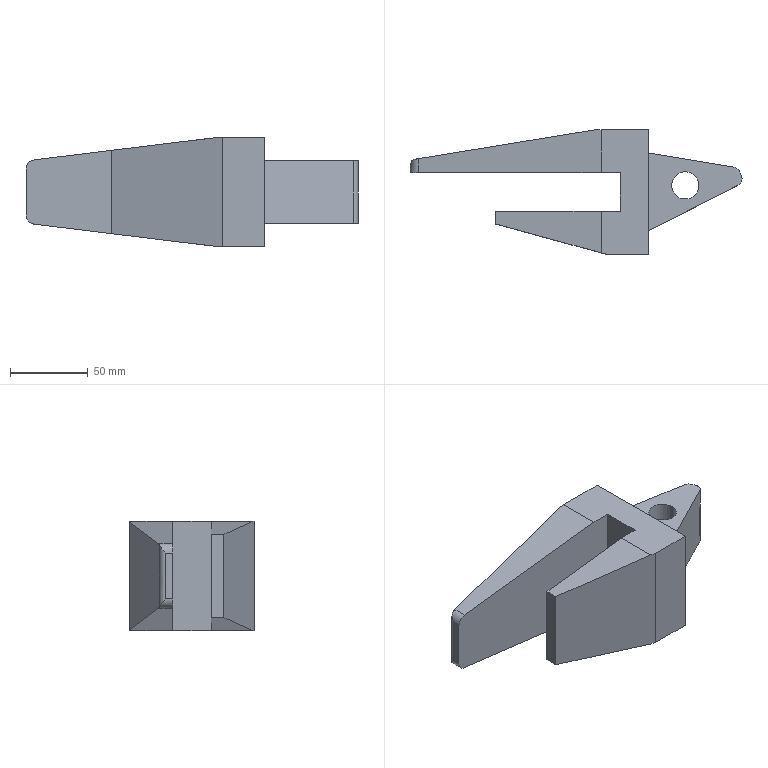Part | SolidWorks | features ICE 2, Extrusion 1, HoleWzd 1 | 1 solid | 29 faces | box 213 x 80 x 70 mm | volume 410977 mm3 | plane 21 | cylinder 8 | commonest cylinder face diameters 10 x3 12 x2 17.5 x2 8 x1
STEP:
#1=CARTESIAN_POINT('',(167.85,44.2,-20.));
#2=VERTEX_POINT('',#1);
#3=CARTESIAN_POINT('',(185.35,44.2,-20.));
#4=VERTEX_POINT('',#3);
#5=CARTESIAN_POINT('',(176.6,44.2,-20.));
#6=DIRECTION('',(0.,0.,1.));
#7=DIRECTION('',(1.,0.,0.));
#8=AXIS2_PLACEMENT_3D('',#5,#6,#7);
#9=CIRCLE('',#8,8.75);
#10=EDGE_CURVE('',#2,#4,#9,.T.);
#11=ORIENTED_EDGE('',*,*,#10,.F.);
#12=CARTESIAN_POINT('',(167.85,44.2,20.));
#13=VERTEX_POINT('',#12);
#14=CARTESIAN_POINT('',(167.85,44.2,20.));
#15=DIRECTION('',(0.,0.,1.));
#16=VECTOR('',#15,1000.);
#17=LINE('',#14,#16);
#18=EDGE_CURVE('',#2,#13,#17,.T.);
#19=ORIENTED_EDGE('',*,*,#18,.T.);
#20=CARTESIAN_POINT('',(185.35,44.2,20.));
#21=VERTEX_POINT('',#20);
#22=CARTESIAN_POINT('',(176.6,44.2,20.));
#23=DIRECTION('',(0.,0.,1.));
#24=DIRECTION('',(1.,0.,0.));
#25=AXIS2_PLACEMENT_3D('',#22,#23,#24);
#26=CIRCLE('',#25,8.75);
#27=EDGE_CURVE('',#13,#21,#26,.T.);
#28=ORIENTED_EDGE('',*,*,#27,.T.);
#29=CARTESIAN_POINT('',(185.35,44.2,20.));
#30=DIRECTION('',(0.,0.,1.));
#31=VECTOR('',#30,1000.);
#32=LINE('',#29,#31);
#33=EDGE_CURVE('',#4,#21,#32,.T.);
#34=ORIENTED_EDGE('',*,*,#33,.F.);
#35=EDGE_LOOP('',(#11,#19,#28,#34));
#36=FACE_OUTER_BOUND('',#35,.T.);
#37=CARTESIAN_POINT('',(176.6,44.2,20.));
#38=DIRECTION('',(0.,0.,1.));
#39=DIRECTION('',(1.,0.,0.));
#40=AXIS2_PLACEMENT_3D('',#37,#38,#39);
#41=CYLINDRICAL_SURFACE('',#40,8.75);
#42=ADVANCED_FACE('',(#36),#41,.F.);
#43=CARTESIAN_POINT('',(210.27,44.18,-20.));
#44=VERTEX_POINT('',#43);
#45=CARTESIAN_POINT('',(213.,48.636,-20.));
#46=VERTEX_POINT('',#45);
#47=CARTESIAN_POINT('',(208.,48.636,-20.));
#48=DIRECTION('',(0.,0.,1.));
#49=DIRECTION('',(1.,0.,0.));
#50=AXIS2_PLACEMENT_3D('',#47,#48,#49);
#51=CIRCLE('',#50,5.);
#52=EDGE_CURVE('',#44,#46,#51,.T.);
#53=ORIENTED_EDGE('',*,*,#52,.T.);
#54=CARTESIAN_POINT('',(213.,48.636,20.));
#55=VERTEX_POINT('',#54);
#56=CARTESIAN_POINT('',(213.,48.636,-20.));
#57=DIRECTION('',(0.,0.,1.));
#58=VECTOR('',#57,1000.);
#59=LINE('',#56,#58);
#60=EDGE_CURVE('',#46,#55,#59,.T.);
#61=ORIENTED_EDGE('',*,*,#60,.T.);
#62=CARTESIAN_POINT('',(210.27,44.18,20.));
#63=VERTEX_POINT('',#62);
#64=CARTESIAN_POINT('',(208.,48.636,20.));
#65=DIRECTION('',(0.,0.,1.));
#66=DIRECTION('',(1.,0.,0.));
#67=AXIS2_PLACEMENT_3D('',#64,#65,#66);
#68=CIRCLE('',#67,5.);
#69=EDGE_CURVE('',#63,#55,#68,.T.);
#70=ORIENTED_EDGE('',*,*,#69,.F.);
#71=CARTESIAN_POINT('',(210.27,44.18,-20.));
#72=DIRECTION('',(0.,0.,1.));
#73=VECTOR('',#72,1000.);
#74=LINE('',#71,#73);
#75=EDGE_CURVE('',#44,#63,#74,.T.);
#76=ORIENTED_EDGE('',*,*,#75,.F.);
#77=EDGE_LOOP('',(#53,#61,#70,#76));
#78=FACE_OUTER_BOUND('',#77,.T.);
#79=CARTESIAN_POINT('',(208.,48.636,-20.));
#80=DIRECTION('',(0.,0.,1.));
#81=DIRECTION('',(1.,0.,0.));
#82=AXIS2_PLACEMENT_3D('',#79,#80,#81);
#83=CYLINDRICAL_SURFACE('',#82,5.);
#84=ADVANCED_FACE('',(#78),#83,.T.);
#85=CARTESIAN_POINT('',(153.,0.,35.));
#86=VERTEX_POINT('',#85);
#87=CARTESIAN_POINT('',(153.,0.,-35.));
#88=VERTEX_POINT('',#87);
#89=CARTESIAN_POINT('',(153.,0.,-35.));
#90=DIRECTION('',(0.,0.,-1.));
#91=VECTOR('',#90,1000.);
#92=LINE('',#89,#91);
#93=EDGE_CURVE('',#86,#88,#92,.T.);
#94=ORIENTED_EDGE('',*,*,#93,.T.);
#95=CARTESIAN_POINT('',(153.,80.,-35.));
#96=VERTEX_POINT('',#95);
#97=CARTESIAN_POINT('',(153.,80.,-35.));
#98=DIRECTION('',(0.,-1.,0.));
#99=VECTOR('',#98,1000.);
#100=LINE('',#97,#99);
#101=EDGE_CURVE('',#96,#88,#100,.T.);
#102=ORIENTED_EDGE('',*,*,#101,.F.);
#103=CARTESIAN_POINT('',(153.,80.,35.));
#104=VERTEX_POINT('',#103);
#105=CARTESIAN_POINT('',(153.,80.,-35.));
#106=DIRECTION('',(0.,0.,-1.));
#107=VECTOR('',#106,1000.);
#108=LINE('',#105,#107);
#109=EDGE_CURVE('',#104,#96,#108,.T.);
#110=ORIENTED_EDGE('',*,*,#109,.F.);
#111=CARTESIAN_POINT('',(153.,80.,35.));
#112=DIRECTION('',(0.,-1.,0.));
#113=VECTOR('',#112,1000.);
#114=LINE('',#111,#113);
#115=EDGE_CURVE('',#104,#86,#114,.T.);
#116=ORIENTED_EDGE('',*,*,#115,.T.);
#117=EDGE_LOOP('',(#94,#102,#110,#116));
#118=FACE_OUTER_BOUND('',#117,.T.);
#119=CARTESIAN_POINT('',(153.,65.,-20.));
#120=VERTEX_POINT('',#119);
#121=CARTESIAN_POINT('',(153.,15.,-20.));
#122=VERTEX_POINT('',#121);
#123=CARTESIAN_POINT('',(153.,65.,-20.));
#124=DIRECTION('',(0.,-1.,0.));
#125=VECTOR('',#124,1000.);
#126=LINE('',#123,#125);
#127=EDGE_CURVE('',#120,#122,#126,.T.);
#128=ORIENTED_EDGE('',*,*,#127,.T.);
#129=CARTESIAN_POINT('',(153.,15.,20.));
#130=VERTEX_POINT('',#129);
#131=CARTESIAN_POINT('',(153.,15.,-20.));
#132=DIRECTION('',(0.,0.,1.));
#133=VECTOR('',#132,1000.);
#134=LINE('',#131,#133);
#135=EDGE_CURVE('',#122,#130,#134,.T.);
#136=ORIENTED_EDGE('',*,*,#135,.T.);
#137=CARTESIAN_POINT('',(153.,65.,20.));
#138=VERTEX_POINT('',#137);
#139=CARTESIAN_POINT('',(153.,65.,20.));
#140=DIRECTION('',(0.,-1.,0.));
#141=VECTOR('',#140,1000.);
#142=LINE('',#139,#141);
#143=EDGE_CURVE('',#138,#130,#142,.T.);
#144=ORIENTED_EDGE('',*,*,#143,.F.);
#145=CARTESIAN_POINT('',(153.,65.,-20.));
#146=DIRECTION('',(0.,0.,1.));
#147=VECTOR('',#146,1000.);
#148=LINE('',#145,#147);
#149=EDGE_CURVE('',#120,#138,#148,.T.);
#150=ORIENTED_EDGE('',*,*,#149,.F.);
#151=EDGE_LOOP('',(#128,#136,#144,#150));
#152=FACE_BOUND('',#151,.T.);
#153=CARTESIAN_POINT('',(153.,80.,-35.));
#154=DIRECTION('',(-1.,0.,0.));
#155=DIRECTION('',(0.,0.,1.));
#156=AXIS2_PLACEMENT_3D('',#153,#154,#155);
#157=PLANE('',#156);
#158=ADVANCED_FACE('',(#118,#152),#157,.F.);
#159=CARTESIAN_POINT('',(122.6,0.9076,-35.));
#160=VERTEX_POINT('',#159);
#161=CARTESIAN_POINT('',(125.9,0.,-35.));
#162=VERTEX_POINT('',#161);
#163=CARTESIAN_POINT('',(55.,19.5,-35.));
#164=DIRECTION('',(0.9642,-0.2652,0.));
#165=VECTOR('',#164,1000.);
#166=LINE('',#163,#165);
#167=EDGE_CURVE('',#160,#162,#166,.T.);
#168=ORIENTED_EDGE('',*,*,#167,.F.);
#169=CARTESIAN_POINT('',(122.6,27.5,-35.));
#170=VERTEX_POINT('',#169);
#171=CARTESIAN_POINT('',(122.6,80.,-35.));
#172=DIRECTION('',(0.,-1.,0.));
#173=VECTOR('',#172,1000.);
#174=LINE('',#171,#173);
#175=EDGE_CURVE('',#170,#160,#174,.T.);
#176=ORIENTED_EDGE('',*,*,#175,.F.);
#177=CARTESIAN_POINT('',(135.,27.5,-35.));
#178=VERTEX_POINT('',#177);
#179=CARTESIAN_POINT('',(55.,27.5,-35.));
#180=DIRECTION('',(1.,0.,0.));
#181=VECTOR('',#180,1000.);
#182=LINE('',#179,#181);
#183=EDGE_CURVE('',#170,#178,#182,.T.);
#184=ORIENTED_EDGE('',*,*,#183,.T.);
#185=CARTESIAN_POINT('',(135.,52.5,-35.));
#186=VERTEX_POINT('',#185);
#187=CARTESIAN_POINT('',(135.,52.5,-35.));
#188=DIRECTION('',(0.,-1.,0.));
#189=VECTOR('',#188,1000.);
#190=LINE('',#187,#189);
#191=EDGE_CURVE('',#186,#178,#190,.T.);
#192=ORIENTED_EDGE('',*,*,#191,.F.);
#193=CARTESIAN_POINT('',(122.6,52.5,-35.));
#194=VERTEX_POINT('',#193);
#195=CARTESIAN_POINT('',(135.,52.5,-35.));
#196=DIRECTION('',(-1.,0.,0.));
#197=VECTOR('',#196,1000.);
#198=LINE('',#195,#197);
#199=EDGE_CURVE('',#186,#194,#198,.T.);
#200=ORIENTED_EDGE('',*,*,#199,.T.);
#201=CARTESIAN_POINT('',(122.6,80.,-35.));
#202=VERTEX_POINT('',#201);
#203=CARTESIAN_POINT('',(122.6,80.,-35.));
#204=DIRECTION('',(0.,-1.,0.));
#205=VECTOR('',#204,1000.);
#206=LINE('',#203,#205);
#207=EDGE_CURVE('',#202,#194,#206,.T.);
#208=ORIENTED_EDGE('',*,*,#207,.F.);
#209=CARTESIAN_POINT('',(153.,80.,-35.));
#210=DIRECTION('',(-1.,0.,0.));
#211=VECTOR('',#210,1000.);
#212=LINE('',#209,#211);
#213=EDGE_CURVE('',#96,#202,#212,.T.);
#214=ORIENTED_EDGE('',*,*,#213,.F.);
#215=ORIENTED_EDGE('',*,*,#101,.T.);
#216=CARTESIAN_POINT('',(153.,0.,-35.));
#217=DIRECTION('',(-1.,0.,0.));
#218=VECTOR('',#217,1000.);
#219=LINE('',#216,#218);
#220=EDGE_CURVE('',#88,#162,#219,.T.);
#221=ORIENTED_EDGE('',*,*,#220,.T.);
#222=EDGE_LOOP('',(#168,#176,#184,#192,#200,#208,#214,#215,#221));
#223=FACE_OUTER_BOUND('',#222,.T.);
#224=CARTESIAN_POINT('',(153.,80.,-35.));
#225=DIRECTION('',(0.,0.,1.));
#226=DIRECTION('',(1.,0.,0.));
#227=AXIS2_PLACEMENT_3D('',#224,#225,#226);
#228=PLANE('',#227);
#229=ADVANCED_FACE('',(#223),#228,.F.);
#230=ORIENTED_EDGE('',*,*,#207,.T.);
#231=CARTESIAN_POINT('',(5.271,52.5,-20.645));
#232=VERTEX_POINT('',#231);
#233=CARTESIAN_POINT('',(122.6,52.5,-35.));
#234=DIRECTION('',(-0.9926,0.,0.1214));
#235=VECTOR('',#234,1000.);
#236=LINE('',#233,#235);
#237=EDGE_CURVE('',#194,#232,#236,.T.);
#238=ORIENTED_EDGE('',*,*,#237,.T.);
#239=CARTESIAN_POINT('',(5.271,61.359,-20.645));
#240=VERTEX_POINT('',#239);
#241=CARTESIAN_POINT('',(5.271,80.,-20.645));
#242=DIRECTION('',(0.,-1.,0.));
#243=VECTOR('',#242,1000.);
#244=LINE('',#241,#243);
#245=EDGE_CURVE('',#240,#232,#244,.T.);
#246=ORIENTED_EDGE('',*,*,#245,.F.);
#247=CARTESIAN_POINT('',(119.6,80.,-34.633));
#248=VERTEX_POINT('',#247);
#249=CARTESIAN_POINT('',(122.523,80.477,-34.991));
#250=DIRECTION('',(0.9798,0.1598,-0.1199));
#251=VECTOR('',#250,1000.);
#252=LINE('',#249,#251);
#253=EDGE_CURVE('',#240,#248,#252,.T.);
#254=ORIENTED_EDGE('',*,*,#253,.T.);
#255=CARTESIAN_POINT('',(122.6,80.,-35.));
#256=DIRECTION('',(-0.9926,0.,0.1214));
#257=VECTOR('',#256,1000.);
#258=LINE('',#255,#257);
#259=EDGE_CURVE('',#202,#248,#258,.T.);
#260=ORIENTED_EDGE('',*,*,#259,.F.);
#261=EDGE_LOOP('',(#230,#238,#246,#254,#260));
#262=FACE_OUTER_BOUND('',#261,.T.);
#263=CARTESIAN_POINT('',(122.6,80.,-35.));
#264=DIRECTION('',(0.1214,0.,0.9926));
#265=DIRECTION('',(0.9926,0.,-0.1214));
#266=AXIS2_PLACEMENT_3D('',#263,#264,#265);
#267=PLANE('',#266);
#268=ADVANCED_FACE('',(#262),#267,.F.);
#269=ORIENTED_EDGE('',*,*,#245,.T.);
#270=CARTESIAN_POINT('',(0.,52.5,-14.689));
#271=VERTEX_POINT('',#270);
#272=CARTESIAN_POINT('',(6.,52.5,-14.689));
#273=DIRECTION('',(0.,1.,0.));
#274=DIRECTION('',(0.,0.,1.));
#275=AXIS2_PLACEMENT_3D('',#272,#273,#274);
#276=CIRCLE('',#275,6.);
#277=EDGE_CURVE('',#232,#271,#276,.T.);
#278=ORIENTED_EDGE('',*,*,#277,.T.);
#279=CARTESIAN_POINT('',(0.,57.099,-14.689));
#280=VERTEX_POINT('',#279);
#281=CARTESIAN_POINT('',(0.,80.,-14.689));
#282=DIRECTION('',(0.,-1.,0.));
#283=VECTOR('',#282,1000.);
#284=LINE('',#281,#283);
#285=EDGE_CURVE('',#280,#271,#284,.T.);
#286=ORIENTED_EDGE('',*,*,#285,.F.);
#287=CARTESIAN_POINT('',(3.356,61.047,-20.076));
#288=VERTEX_POINT('',#287);
#289=CARTESIAN_POINT('',(0.,57.099,-14.689));
#290=CARTESIAN_POINT('',(0.,57.515,-15.198));
#291=CARTESIAN_POINT('',(0.06502,57.932,-15.709));
#292=CARTESIAN_POINT('',(0.3252,58.735,-16.705));
#293=CARTESIAN_POINT('',(0.5188,59.121,-17.19));
#294=CARTESIAN_POINT('',(0.925,59.668,-17.902));
#295=CARTESIAN_POINT('',(1.08,59.843,-18.135));
#296=CARTESIAN_POINT('',(1.425,60.17,-18.582));
#297=CARTESIAN_POINT('',(1.617,60.322,-18.797));
#298=CARTESIAN_POINT('',(2.044,60.598,-19.211));
#299=CARTESIAN_POINT('',(2.282,60.722,-19.409));
#300=CARTESIAN_POINT('',(2.789,60.921,-19.768));
#301=CARTESIAN_POINT('',(3.062,60.999,-19.931));
#302=CARTESIAN_POINT('',(3.356,61.047,-20.076));
#303=B_SPLINE_CURVE_WITH_KNOTS('',3,(#289,#290,#291,#292,#293,#294,#295,#296,#297,#298,#299,#300,#301,#302),.UNSPECIFIED.,.F.,.F.,(4,2,2,2,2,2,4),(-0.00001549,0.001955,0.003925,0.00491,0.005895,0.00688,0.007865),.UNSPECIFIED.);
#304=EDGE_CURVE('',#280,#288,#303,.T.);
#305=ORIENTED_EDGE('',*,*,#304,.T.);
#306=CARTESIAN_POINT('',(3.356,61.047,-20.076));
#307=CARTESIAN_POINT('',(3.96,61.146,-20.372));
#308=CARTESIAN_POINT('',(4.604,61.251,-20.563));
#309=CARTESIAN_POINT('',(5.271,61.359,-20.645));
#310=(BOUNDED_CURVE()B_SPLINE_CURVE(3,(#306,#307,#308,#309),.UNSPECIFIED.,.F.,.F.)B_SPLINE_CURVE_WITH_KNOTS((4,4),(1.115,1.449),.UNSPECIFIED.)CURVE()GEOMETRIC_REPRESENTATION_ITEM()RATIONAL_B_SPLINE_CURVE((1.,0.9907,0.9907,1.))REPRESENTATION_ITEM(''));
#311=EDGE_CURVE('',#288,#240,#310,.T.);
#312=ORIENTED_EDGE('',*,*,#311,.T.);
#313=EDGE_LOOP('',(#269,#278,#286,#305,#312));
#314=FACE_OUTER_BOUND('',#313,.T.);
#315=CARTESIAN_POINT('',(6.,80.,-14.689));
#316=DIRECTION('',(0.,-1.,0.));
#317=DIRECTION('',(0.,0.,-1.));
#318=AXIS2_PLACEMENT_3D('',#315,#316,#317);
#319=CYLINDRICAL_SURFACE('',#318,6.);
#320=ADVANCED_FACE('',(#314),#319,.T.);
#321=ORIENTED_EDGE('',*,*,#285,.T.);
#322=CARTESIAN_POINT('',(0.,52.5,14.689));
#323=VERTEX_POINT('',#322);
#324=CARTESIAN_POINT('',(0.,52.5,-35.));
#325=DIRECTION('',(0.,0.,1.));
#326=VECTOR('',#325,1000.);
#327=LINE('',#324,#326);
#328=EDGE_CURVE('',#271,#323,#327,.T.);
#329=ORIENTED_EDGE('',*,*,#328,.T.);
#330=CARTESIAN_POINT('',(0.,57.099,14.689));
#331=VERTEX_POINT('',#330);
#332=CARTESIAN_POINT('',(0.,80.,14.689));
#333=DIRECTION('',(0.,-1.,0.));
#334=VECTOR('',#333,1000.);
#335=LINE('',#332,#334);
#336=EDGE_CURVE('',#331,#323,#335,.T.);
#337=ORIENTED_EDGE('',*,*,#336,.F.);
#338=CARTESIAN_POINT('',(0.,57.099,-35.));
#339=DIRECTION('',(0.,0.,1.));
#340=VECTOR('',#339,1000.);
#341=LINE('',#338,#340);
#342=EDGE_CURVE('',#280,#331,#341,.T.);
#343=ORIENTED_EDGE('',*,*,#342,.F.);
#344=EDGE_LOOP('',(#321,#329,#337,#343));
#345=FACE_OUTER_BOUND('',#344,.T.);
#346=CARTESIAN_POINT('',(0.,80.,-14.689));
#347=DIRECTION('',(1.,0.,0.));
#348=DIRECTION('',(0.,0.,-1.));
#349=AXIS2_PLACEMENT_3D('',#346,#347,#348);
#350=PLANE('',#349);
#351=ADVANCED_FACE('',(#345),#350,.F.);
#352=ORIENTED_EDGE('',*,*,#336,.T.);
#353=CARTESIAN_POINT('',(5.271,52.5,20.645));
#354=VERTEX_POINT('',#353);
#355=CARTESIAN_POINT('',(6.,52.5,14.689));
#356=DIRECTION('',(0.,1.,0.));
#357=DIRECTION('',(0.,0.,1.));
#358=AXIS2_PLACEMENT_3D('',#355,#356,#357);
#359=CIRCLE('',#358,6.);
#360=EDGE_CURVE('',#323,#354,#359,.T.);
#361=ORIENTED_EDGE('',*,*,#360,.T.);
#362=CARTESIAN_POINT('',(5.271,61.359,20.645));
#363=VERTEX_POINT('',#362);
#364=CARTESIAN_POINT('',(5.271,80.,20.645));
#365=DIRECTION('',(0.,-1.,0.));
#366=VECTOR('',#365,1000.);
#367=LINE('',#364,#366);
#368=EDGE_CURVE('',#363,#354,#367,.T.);
#369=ORIENTED_EDGE('',*,*,#368,.F.);
#370=CARTESIAN_POINT('',(3.356,61.047,20.076));
#371=VERTEX_POINT('',#370);
#372=CARTESIAN_POINT('',(5.271,61.359,20.645));
#373=CARTESIAN_POINT('',(4.604,61.251,20.563));
#374=CARTESIAN_POINT('',(3.96,61.146,20.372));
#375=CARTESIAN_POINT('',(3.356,61.047,20.076));
#376=(BOUNDED_CURVE()B_SPLINE_CURVE(3,(#372,#373,#374,#375),.UNSPECIFIED.,.F.,.F.)B_SPLINE_CURVE_WITH_KNOTS((4,4),(4.834,5.169),.UNSPECIFIED.)CURVE()GEOMETRIC_REPRESENTATION_ITEM()RATIONAL_B_SPLINE_CURVE((1.,0.9907,0.9907,1.))REPRESENTATION_ITEM(''));
#377=EDGE_CURVE('',#363,#371,#376,.T.);
#378=ORIENTED_EDGE('',*,*,#377,.T.);
#379=CARTESIAN_POINT('',(3.356,61.047,20.076));
#380=CARTESIAN_POINT('',(3.062,60.999,19.931));
#381=CARTESIAN_POINT('',(2.789,60.921,19.768));
#382=CARTESIAN_POINT('',(2.282,60.722,19.409));
#383=CARTESIAN_POINT('',(2.044,60.598,19.211));
#384=CARTESIAN_POINT('',(1.617,60.322,18.797));
#385=CARTESIAN_POINT('',(1.425,60.17,18.582));
#386=CARTESIAN_POINT('',(1.08,59.843,18.135));
#387=CARTESIAN_POINT('',(0.925,59.668,17.902));
#388=CARTESIAN_POINT('',(0.5188,59.121,17.19));
#389=CARTESIAN_POINT('',(0.3252,58.735,16.705));
#390=CARTESIAN_POINT('',(0.1301,58.133,15.958));
#391=CARTESIAN_POINT('',(0.08113,57.928,15.705));
#392=CARTESIAN_POINT('',(0.0324,57.618,15.325));
#393=CARTESIAN_POINT('',(0.02025,57.515,15.198));
#394=CARTESIAN_POINT('',(0.004051,57.307,14.944));
#395=CARTESIAN_POINT('',(0.,57.203,14.816));
#396=CARTESIAN_POINT('',(0.,57.099,14.689));
#397=B_SPLINE_CURVE_WITH_KNOTS('',3,(#379,#380,#381,#382,#383,#384,#385,#386,#387,#388,#389,#390,#391,#392,#393,#394,#395,#396),.UNSPECIFIED.,.F.,.F.,(4,2,2,2,2,2,2,2,4),(0.,0.0009787,0.001957,0.002936,0.003915,0.005872,0.006851,0.00734,0.007829),.UNSPECIFIED.);
#398=EDGE_CURVE('',#371,#331,#397,.T.);
#399=ORIENTED_EDGE('',*,*,#398,.T.);
#400=EDGE_LOOP('',(#352,#361,#369,#378,#399));
#401=FACE_OUTER_BOUND('',#400,.T.);
#402=CARTESIAN_POINT('',(6.,80.,14.689));
#403=DIRECTION('',(0.,-1.,0.));
#404=DIRECTION('',(0.,0.,-1.));
#405=AXIS2_PLACEMENT_3D('',#402,#403,#404);
#406=CYLINDRICAL_SURFACE('',#405,6.);
#407=ADVANCED_FACE('',(#401),#406,.T.);
#408=ORIENTED_EDGE('',*,*,#368,.T.);
#409=CARTESIAN_POINT('',(122.6,52.5,35.));
#410=VERTEX_POINT('',#409);
#411=CARTESIAN_POINT('',(5.271,52.5,20.645));
#412=DIRECTION('',(0.9926,0.,0.1214));
#413=VECTOR('',#412,1000.);
#414=LINE('',#411,#413);
#415=EDGE_CURVE('',#354,#410,#414,.T.);
#416=ORIENTED_EDGE('',*,*,#415,.T.);
#417=CARTESIAN_POINT('',(122.6,80.,35.));
#418=VERTEX_POINT('',#417);
#419=CARTESIAN_POINT('',(122.6,80.,35.));
#420=DIRECTION('',(0.,-1.,0.));
#421=VECTOR('',#420,1000.);
#422=LINE('',#419,#421);
#423=EDGE_CURVE('',#418,#410,#422,.T.);
#424=ORIENTED_EDGE('',*,*,#423,.F.);
#425=CARTESIAN_POINT('',(119.6,80.,34.633));
#426=VERTEX_POINT('',#425);
#427=CARTESIAN_POINT('',(5.271,80.,20.645));
#428=DIRECTION('',(0.9926,0.,0.1214));
#429=VECTOR('',#428,1000.);
#430=LINE('',#427,#429);
#431=EDGE_CURVE('',#426,#418,#430,.T.);
#432=ORIENTED_EDGE('',*,*,#431,.F.);
#433=CARTESIAN_POINT('',(8.189,61.835,21.002));
#434=DIRECTION('',(-0.9798,-0.1598,-0.1199));
#435=VECTOR('',#434,1000.);
#436=LINE('',#433,#435);
#437=EDGE_CURVE('',#426,#363,#436,.T.);
#438=ORIENTED_EDGE('',*,*,#437,.T.);
#439=EDGE_LOOP('',(#408,#416,#424,#432,#438));
#440=FACE_OUTER_BOUND('',#439,.T.);
#441=CARTESIAN_POINT('',(5.271,80.,20.645));
#442=DIRECTION('',(0.1214,0.,-0.9926));
#443=DIRECTION('',(-0.9926,0.,-0.1214));
#444=AXIS2_PLACEMENT_3D('',#441,#442,#443);
#445=PLANE('',#444);
#446=ADVANCED_FACE('',(#440),#445,.F.);
#447=CARTESIAN_POINT('',(122.6,0.9076,35.));
#448=VERTEX_POINT('',#447);
#449=CARTESIAN_POINT('',(125.9,0.,35.));
#450=VERTEX_POINT('',#449);
#451=CARTESIAN_POINT('',(55.,19.5,35.));
#452=DIRECTION('',(0.9642,-0.2652,0.));
#453=VECTOR('',#452,1000.);
#454=LINE('',#451,#453);
#455=EDGE_CURVE('',#448,#450,#454,.T.);
#456=ORIENTED_EDGE('',*,*,#455,.T.);
#457=CARTESIAN_POINT('',(122.6,0.,35.));
#458=DIRECTION('',(1.,0.,0.));
#459=VECTOR('',#458,1000.);
#460=LINE('',#457,#459);
#461=EDGE_CURVE('',#450,#86,#460,.T.);
#462=ORIENTED_EDGE('',*,*,#461,.T.);
#463=ORIENTED_EDGE('',*,*,#115,.F.);
#464=CARTESIAN_POINT('',(122.6,80.,35.));
#465=DIRECTION('',(1.,0.,0.));
#466=VECTOR('',#465,1000.);
#467=LINE('',#464,#466);
#468=EDGE_CURVE('',#418,#104,#467,.T.);
#469=ORIENTED_EDGE('',*,*,#468,.F.);
#470=ORIENTED_EDGE('',*,*,#423,.T.);
#471=CARTESIAN_POINT('',(135.,52.5,35.));
#472=VERTEX_POINT('',#471);
#473=CARTESIAN_POINT('',(135.,52.5,35.));
#474=DIRECTION('',(-1.,0.,0.));
#475=VECTOR('',#474,1000.);
#476=LINE('',#473,#475);
#477=EDGE_CURVE('',#472,#410,#476,.T.);
#478=ORIENTED_EDGE('',*,*,#477,.F.);
#479=CARTESIAN_POINT('',(135.,27.5,35.));
#480=VERTEX_POINT('',#479);
#481=CARTESIAN_POINT('',(135.,52.5,35.));
#482=DIRECTION('',(0.,-1.,0.));
#483=VECTOR('',#482,1000.);
#484=LINE('',#481,#483);
#485=EDGE_CURVE('',#472,#480,#484,.T.);
#486=ORIENTED_EDGE('',*,*,#485,.T.);
#487=CARTESIAN_POINT('',(122.6,27.5,35.));
#488=VERTEX_POINT('',#487);
#489=CARTESIAN_POINT('',(55.,27.5,35.));
#490=DIRECTION('',(1.,0.,0.));
#491=VECTOR('',#490,1000.);
#492=LINE('',#489,#491);
#493=EDGE_CURVE('',#488,#480,#492,.T.);
#494=ORIENTED_EDGE('',*,*,#493,.F.);
#495=CARTESIAN_POINT('',(122.6,80.,35.));
#496=DIRECTION('',(0.,-1.,0.));
#497=VECTOR('',#496,1000.);
#498=LINE('',#495,#497);
#499=EDGE_CURVE('',#488,#448,#498,.T.);
#500=ORIENTED_EDGE('',*,*,#499,.T.);
#501=EDGE_LOOP('',(#456,#462,#463,#469,#470,#478,#486,#494,#500));
#502=FACE_OUTER_BOUND('',#501,.T.);
#503=CARTESIAN_POINT('',(122.6,80.,35.));
#504=DIRECTION('',(0.,0.,-1.));
#505=DIRECTION('',(-1.,0.,0.));
#506=AXIS2_PLACEMENT_3D('',#503,#504,#505);
#507=PLANE('',#506);
#508=ADVANCED_FACE('',(#502),#507,.F.);
#509=ORIENTED_EDGE('',*,*,#259,.T.);
#510=CARTESIAN_POINT('',(119.6,80.,-14.689));
#511=DIRECTION('',(0.,0.,1.));
#512=VECTOR('',#511,1000.);
#513=LINE('',#510,#512);
#514=EDGE_CURVE('',#248,#426,#513,.T.);
#515=ORIENTED_EDGE('',*,*,#514,.T.);
#516=ORIENTED_EDGE('',*,*,#431,.T.);
#517=ORIENTED_EDGE('',*,*,#468,.T.);
#518=ORIENTED_EDGE('',*,*,#109,.T.);
#519=ORIENTED_EDGE('',*,*,#213,.T.);
#520=EDGE_LOOP('',(#509,#515,#516,#517,#518,#519));
#521=FACE_OUTER_BOUND('',#520,.T.);
#522=CARTESIAN_POINT('',(6.,80.,-14.689));
#523=DIRECTION('',(0.,-1.,0.));
#524=DIRECTION('',(0.,0.,-1.));
#525=AXIS2_PLACEMENT_3D('',#522,#523,#524);
#526=PLANE('',#525);
#527=ADVANCED_FACE('',(#521),#526,.F.);
#528=CARTESIAN_POINT('',(55.,19.5,-26.729));
#529=VERTEX_POINT('',#528);
#530=CARTESIAN_POINT('',(102.654,6.393,-32.56));
#531=DIRECTION('',(0.9576,-0.2634,-0.1172));
#532=VECTOR('',#531,1000.);
#533=LINE('',#530,#532);
#534=EDGE_CURVE('',#529,#160,#533,.T.);
#535=ORIENTED_EDGE('',*,*,#534,.F.);
#536=CARTESIAN_POINT('',(55.,27.5,-26.729));
#537=VERTEX_POINT('',#536);
#538=CARTESIAN_POINT('',(55.,80.,-26.729));
#539=DIRECTION('',(0.,-1.,0.));
#540=VECTOR('',#539,1000.);
#541=LINE('',#538,#540);
#542=EDGE_CURVE('',#537,#529,#541,.T.);
#543=ORIENTED_EDGE('',*,*,#542,.F.);
#544=CARTESIAN_POINT('',(122.6,27.5,-35.));
#545=DIRECTION('',(0.9926,0.,-0.1214));
#546=VECTOR('',#545,1000.);
#547=LINE('',#544,#546);
#548=EDGE_CURVE('',#537,#170,#547,.T.);
#549=ORIENTED_EDGE('',*,*,#548,.T.);
#550=ORIENTED_EDGE('',*,*,#175,.T.);
#551=EDGE_LOOP('',(#535,#543,#549,#550));
#552=FACE_OUTER_BOUND('',#551,.T.);
#553=CARTESIAN_POINT('',(122.6,80.,-35.));
#554=DIRECTION('',(0.1214,0.,0.9926));
#555=DIRECTION('',(0.9926,0.,-0.1214));
#556=AXIS2_PLACEMENT_3D('',#553,#554,#555);
#557=PLANE('',#556);
#558=ADVANCED_FACE('',(#552),#557,.F.);
#559=CARTESIAN_POINT('',(55.,19.5,26.729));
#560=VERTEX_POINT('',#559);
#561=CARTESIAN_POINT('',(-6.537,36.425,19.2));
#562=DIRECTION('',(-0.9576,0.2634,-0.1172));
#563=VECTOR('',#562,1000.);
#564=LINE('',#561,#563);
#565=EDGE_CURVE('',#448,#560,#564,.T.);
#566=ORIENTED_EDGE('',*,*,#565,.F.);
#567=ORIENTED_EDGE('',*,*,#499,.F.);
#568=CARTESIAN_POINT('',(55.,27.5,26.729));
#569=VERTEX_POINT('',#568);
#570=CARTESIAN_POINT('',(5.271,27.5,20.645));
#571=DIRECTION('',(-0.9926,0.,-0.1214));
#572=VECTOR('',#571,1000.);
#573=LINE('',#570,#572);
#574=EDGE_CURVE('',#488,#569,#573,.T.);
#575=ORIENTED_EDGE('',*,*,#574,.T.);
#576=CARTESIAN_POINT('',(55.,80.,26.729));
#577=DIRECTION('',(0.,1.,0.));
#578=VECTOR('',#577,1000.);
#579=LINE('',#576,#578);
#580=EDGE_CURVE('',#560,#569,#579,.T.);
#581=ORIENTED_EDGE('',*,*,#580,.F.);
#582=EDGE_LOOP('',(#566,#567,#575,#581));
#583=FACE_OUTER_BOUND('',#582,.T.);
#584=CARTESIAN_POINT('',(5.271,80.,20.645));
#585=DIRECTION('',(0.1214,0.,-0.9926));
#586=DIRECTION('',(-0.9926,0.,-0.1214));
#587=AXIS2_PLACEMENT_3D('',#584,#585,#586);
#588=PLANE('',#587);
#589=ADVANCED_FACE('',(#583),#588,.F.);
#590=ORIENTED_EDGE('',*,*,#461,.F.);
#591=CARTESIAN_POINT('',(125.9,0.,-35.));
#592=DIRECTION('',(0.,0.,1.));
#593=VECTOR('',#592,1000.);
#594=LINE('',#591,#593);
#595=EDGE_CURVE('',#162,#450,#594,.T.);
#596=ORIENTED_EDGE('',*,*,#595,.F.);
#597=ORIENTED_EDGE('',*,*,#220,.F.);
#598=ORIENTED_EDGE('',*,*,#93,.F.);
#599=EDGE_LOOP('',(#590,#596,#597,#598));
#600=FACE_OUTER_BOUND('',#599,.T.);
#601=CARTESIAN_POINT('',(6.,0.,-14.689));
#602=DIRECTION('',(0.,-1.,0.));
#603=DIRECTION('',(0.,0.,-1.));
#604=AXIS2_PLACEMENT_3D('',#601,#602,#603);
#605=PLANE('',#604);
#606=ADVANCED_FACE('',(#600),#605,.T.);
#607=CARTESIAN_POINT('',(55.,19.5,-35.));
#608=DIRECTION('',(0.,0.,1.));
#609=VECTOR('',#608,1000.);
#610=LINE('',#607,#609);
#611=EDGE_CURVE('',#529,#560,#610,.T.);
#612=ORIENTED_EDGE('',*,*,#611,.F.);
#613=ORIENTED_EDGE('',*,*,#534,.T.);
#614=ORIENTED_EDGE('',*,*,#167,.T.);
#615=ORIENTED_EDGE('',*,*,#595,.T.);
#616=ORIENTED_EDGE('',*,*,#455,.F.);
#617=ORIENTED_EDGE('',*,*,#565,.T.);
#618=EDGE_LOOP('',(#612,#613,#614,#615,#616,#617));
#619=FACE_OUTER_BOUND('',#618,.T.);
#620=CARTESIAN_POINT('',(55.,19.5,-35.));
#621=DIRECTION('',(-0.2652,-0.9642,0.));
#622=DIRECTION('',(0.9642,-0.2652,0.));
#623=AXIS2_PLACEMENT_3D('',#620,#621,#622);
#624=PLANE('',#623);
#625=ADVANCED_FACE('',(#619),#624,.T.);
#626=CARTESIAN_POINT('',(135.,27.5,-35.));
#627=DIRECTION('',(0.,0.,1.));
#628=VECTOR('',#627,1000.);
#629=LINE('',#626,#628);
#630=EDGE_CURVE('',#178,#480,#629,.T.);
#631=ORIENTED_EDGE('',*,*,#630,.T.);
#632=ORIENTED_EDGE('',*,*,#485,.F.);
#633=CARTESIAN_POINT('',(135.,52.5,-35.));
#634=DIRECTION('',(0.,0.,1.));
#635=VECTOR('',#634,1000.);
#636=LINE('',#633,#635);
#637=EDGE_CURVE('',#186,#472,#636,.T.);
#638=ORIENTED_EDGE('',*,*,#637,.F.);
#639=ORIENTED_EDGE('',*,*,#191,.T.);
#640=EDGE_LOOP('',(#631,#632,#638,#639));
#641=FACE_OUTER_BOUND('',#640,.T.);
#642=CARTESIAN_POINT('',(135.,52.5,-35.));
#643=DIRECTION('',(-1.,0.,0.));
#644=DIRECTION('',(0.,-1.,0.));
#645=AXIS2_PLACEMENT_3D('',#642,#643,#644);
#646=PLANE('',#645);
#647=ADVANCED_FACE('',(#641),#646,.T.);
#648=ORIENTED_EDGE('',*,*,#548,.F.);
#649=CARTESIAN_POINT('',(55.,27.5,-35.));
#650=DIRECTION('',(0.,0.,1.));
#651=VECTOR('',#650,1000.);
#652=LINE('',#649,#651);
#653=EDGE_CURVE('',#537,#569,#652,.T.);
#654=ORIENTED_EDGE('',*,*,#653,.T.);
#655=ORIENTED_EDGE('',*,*,#574,.F.);
#656=ORIENTED_EDGE('',*,*,#493,.T.);
#657=ORIENTED_EDGE('',*,*,#630,.F.);
#658=ORIENTED_EDGE('',*,*,#183,.F.);
#659=EDGE_LOOP('',(#648,#654,#655,#656,#657,#658));
#660=FACE_OUTER_BOUND('',#659,.T.);
#661=CARTESIAN_POINT('',(55.,27.5,-35.));
#662=DIRECTION('',(0.,-1.,0.));
#663=DIRECTION('',(0.,0.,-1.));
#664=AXIS2_PLACEMENT_3D('',#661,#662,#663);
#665=PLANE('',#664);
#666=ADVANCED_FACE('',(#660),#665,.F.);
#667=ORIENTED_EDGE('',*,*,#237,.F.);
#668=ORIENTED_EDGE('',*,*,#199,.F.);
#669=ORIENTED_EDGE('',*,*,#637,.T.);
#670=ORIENTED_EDGE('',*,*,#477,.T.);
#671=ORIENTED_EDGE('',*,*,#415,.F.);
#672=ORIENTED_EDGE('',*,*,#360,.F.);
#673=ORIENTED_EDGE('',*,*,#328,.F.);
#674=ORIENTED_EDGE('',*,*,#277,.F.);
#675=EDGE_LOOP('',(#667,#668,#669,#670,#671,#672,#673,#674));
#676=FACE_OUTER_BOUND('',#675,.T.);
#677=CARTESIAN_POINT('',(135.,52.5,-35.));
#678=DIRECTION('',(0.,1.,0.));
#679=DIRECTION('',(0.,0.,1.));
#680=AXIS2_PLACEMENT_3D('',#677,#678,#679);
#681=PLANE('',#680);
#682=ADVANCED_FACE('',(#676),#681,.F.);
#683=ORIENTED_EDGE('',*,*,#653,.F.);
#684=ORIENTED_EDGE('',*,*,#542,.T.);
#685=ORIENTED_EDGE('',*,*,#611,.T.);
#686=ORIENTED_EDGE('',*,*,#580,.T.);
#687=EDGE_LOOP('',(#683,#684,#685,#686));
#688=FACE_OUTER_BOUND('',#687,.T.);
#689=CARTESIAN_POINT('',(55.,27.5,-35.));
#690=DIRECTION('',(-1.,0.,0.));
#691=DIRECTION('',(0.,0.,1.));
#692=AXIS2_PLACEMENT_3D('',#689,#690,#691);
#693=PLANE('',#692);
#694=ADVANCED_FACE('',(#688),#693,.T.);
#695=ORIENTED_EDGE('',*,*,#304,.F.);
#696=ORIENTED_EDGE('',*,*,#342,.T.);
#697=ORIENTED_EDGE('',*,*,#398,.F.);
#698=CARTESIAN_POINT('',(3.356,61.047,-35.));
#699=DIRECTION('',(0.,0.,1.));
#700=VECTOR('',#699,1000.);
#701=LINE('',#698,#700);
#702=EDGE_CURVE('',#288,#371,#701,.T.);
#703=ORIENTED_EDGE('',*,*,#702,.F.);
#704=EDGE_LOOP('',(#695,#696,#697,#703));
#705=FACE_OUTER_BOUND('',#704,.T.);
#706=CARTESIAN_POINT('',(4.,57.099,-35.));
#707=DIRECTION('',(0.,0.,1.));
#708=DIRECTION('',(1.,0.,0.));
#709=AXIS2_PLACEMENT_3D('',#706,#707,#708);
#710=CYLINDRICAL_SURFACE('',#709,4.);
#711=ADVANCED_FACE('',(#705),#710,.T.);
#712=ORIENTED_EDGE('',*,*,#253,.F.);
#713=ORIENTED_EDGE('',*,*,#311,.F.);
#714=ORIENTED_EDGE('',*,*,#702,.T.);
#715=ORIENTED_EDGE('',*,*,#377,.F.);
#716=ORIENTED_EDGE('',*,*,#437,.F.);
#717=ORIENTED_EDGE('',*,*,#514,.F.);
#718=EDGE_LOOP('',(#712,#713,#714,#715,#716,#717));
#719=FACE_OUTER_BOUND('',#718,.T.);
#720=CARTESIAN_POINT('',(3.356,61.047,-35.));
#721=DIRECTION('',(0.1609,-0.987,0.));
#722=DIRECTION('',(0.987,0.1609,0.));
#723=AXIS2_PLACEMENT_3D('',#720,#721,#722);
#724=PLANE('',#723);
#725=ADVANCED_FACE('',(#719),#724,.F.);
#726=ORIENTED_EDGE('',*,*,#75,.T.);
#727=CARTESIAN_POINT('',(153.,15.,20.));
#728=DIRECTION('',(0.891,0.454,0.));
#729=VECTOR('',#728,1000.);
#730=LINE('',#727,#729);
#731=EDGE_CURVE('',#130,#63,#730,.T.);
#732=ORIENTED_EDGE('',*,*,#731,.F.);
#733=ORIENTED_EDGE('',*,*,#135,.F.);
#734=CARTESIAN_POINT('',(153.,15.,-20.));
#735=DIRECTION('',(0.891,0.454,0.));
#736=VECTOR('',#735,1000.);
#737=LINE('',#734,#736);
#738=EDGE_CURVE('',#122,#44,#737,.T.);
#739=ORIENTED_EDGE('',*,*,#738,.T.);
#740=EDGE_LOOP('',(#726,#732,#733,#739));
#741=FACE_OUTER_BOUND('',#740,.T.);
#742=CARTESIAN_POINT('',(153.,15.,-20.));
#743=DIRECTION('',(0.454,-0.891,0.));
#744=DIRECTION('',(0.891,0.454,0.));
#745=AXIS2_PLACEMENT_3D('',#742,#743,#744);
#746=PLANE('',#745);
#747=ADVANCED_FACE('',(#741),#746,.T.);
#748=ORIENTED_EDGE('',*,*,#149,.T.);
#749=CARTESIAN_POINT('',(207.838,55.922,20.));
#750=VERTEX_POINT('',#749);
#751=CARTESIAN_POINT('',(207.838,55.922,20.));
#752=DIRECTION('',(-0.9866,0.1633,0.));
#753=VECTOR('',#752,1000.);
#754=LINE('',#751,#753);
#755=EDGE_CURVE('',#750,#138,#754,.T.);
#756=ORIENTED_EDGE('',*,*,#755,.F.);
#757=CARTESIAN_POINT('',(207.838,55.922,-20.));
#758=VERTEX_POINT('',#757);
#759=CARTESIAN_POINT('',(207.838,55.922,-20.));
#760=DIRECTION('',(0.,0.,1.));
#761=VECTOR('',#760,1000.);
#762=LINE('',#759,#761);
#763=EDGE_CURVE('',#758,#750,#762,.T.);
#764=ORIENTED_EDGE('',*,*,#763,.F.);
#765=CARTESIAN_POINT('',(207.838,55.922,-20.));
#766=DIRECTION('',(-0.9866,0.1633,0.));
#767=VECTOR('',#766,1000.);
#768=LINE('',#765,#767);
#769=EDGE_CURVE('',#758,#120,#768,.T.);
#770=ORIENTED_EDGE('',*,*,#769,.T.);
#771=EDGE_LOOP('',(#748,#756,#764,#770));
#772=FACE_OUTER_BOUND('',#771,.T.);
#773=CARTESIAN_POINT('',(207.838,55.922,-20.));
#774=DIRECTION('',(0.1633,0.9866,0.));
#775=DIRECTION('',(-0.9866,0.1633,0.));
#776=AXIS2_PLACEMENT_3D('',#773,#774,#775);
#777=PLANE('',#776);
#778=ADVANCED_FACE('',(#772),#777,.T.);
#779=ORIENTED_EDGE('',*,*,#763,.T.);
#780=CARTESIAN_POINT('',(211.638,52.909,20.));
#781=VERTEX_POINT('',#780);
#782=CARTESIAN_POINT('',(207.021,50.989,20.));
#783=DIRECTION('',(0.,0.,1.));
#784=DIRECTION('',(-1.,0.,0.));
#785=AXIS2_PLACEMENT_3D('',#782,#783,#784);
#786=CIRCLE('',#785,5.);
#787=EDGE_CURVE('',#781,#750,#786,.T.);
#788=ORIENTED_EDGE('',*,*,#787,.F.);
#789=CARTESIAN_POINT('',(211.638,52.909,-20.));
#790=VERTEX_POINT('',#789);
#791=CARTESIAN_POINT('',(211.638,52.909,-20.));
#792=DIRECTION('',(0.,0.,1.));
#793=VECTOR('',#792,1000.);
#794=LINE('',#791,#793);
#795=EDGE_CURVE('',#790,#781,#794,.T.);
#796=ORIENTED_EDGE('',*,*,#795,.F.);
#797=CARTESIAN_POINT('',(207.021,50.989,-20.));
#798=DIRECTION('',(0.,0.,1.));
#799=DIRECTION('',(-1.,0.,0.));
#800=AXIS2_PLACEMENT_3D('',#797,#798,#799);
#801=CIRCLE('',#800,5.);
#802=EDGE_CURVE('',#790,#758,#801,.T.);
#803=ORIENTED_EDGE('',*,*,#802,.T.);
#804=EDGE_LOOP('',(#779,#788,#796,#803));
#805=FACE_OUTER_BOUND('',#804,.T.);
#806=CARTESIAN_POINT('',(207.021,50.989,-20.));
#807=DIRECTION('',(0.,0.,1.));
#808=DIRECTION('',(1.,0.,0.));
#809=AXIS2_PLACEMENT_3D('',#806,#807,#808);
#810=CYLINDRICAL_SURFACE('',#809,5.);
#811=ADVANCED_FACE('',(#805),#810,.T.);
#812=ORIENTED_EDGE('',*,*,#795,.T.);
#813=CARTESIAN_POINT('',(212.617,50.556,20.));
#814=VERTEX_POINT('',#813);
#815=CARTESIAN_POINT('',(212.617,50.556,20.));
#816=DIRECTION('',(-0.384,0.9233,0.));
#817=VECTOR('',#816,1000.);
#818=LINE('',#815,#817);
#819=EDGE_CURVE('',#814,#781,#818,.T.);
#820=ORIENTED_EDGE('',*,*,#819,.F.);
#821=CARTESIAN_POINT('',(212.617,50.556,-20.));
#822=VERTEX_POINT('',#821);
#823=CARTESIAN_POINT('',(212.617,50.556,-20.));
#824=DIRECTION('',(0.,0.,1.));
#825=VECTOR('',#824,1000.);
#826=LINE('',#823,#825);
#827=EDGE_CURVE('',#822,#814,#826,.T.);
#828=ORIENTED_EDGE('',*,*,#827,.F.);
#829=CARTESIAN_POINT('',(212.617,50.556,-20.));
#830=DIRECTION('',(-0.384,0.9233,0.));
#831=VECTOR('',#830,1000.);
#832=LINE('',#829,#831);
#833=EDGE_CURVE('',#822,#790,#832,.T.);
#834=ORIENTED_EDGE('',*,*,#833,.T.);
#835=EDGE_LOOP('',(#812,#820,#828,#834));
#836=FACE_OUTER_BOUND('',#835,.T.);
#837=CARTESIAN_POINT('',(212.617,50.556,-20.));
#838=DIRECTION('',(0.9233,0.384,0.));
#839=DIRECTION('',(-0.384,0.9233,0.));
#840=AXIS2_PLACEMENT_3D('',#837,#838,#839);
#841=PLANE('',#840);
#842=ADVANCED_FACE('',(#836),#841,.T.);
#843=ORIENTED_EDGE('',*,*,#60,.F.);
#844=CARTESIAN_POINT('',(208.,48.636,-20.));
#845=DIRECTION('',(0.,0.,1.));
#846=DIRECTION('',(1.,0.,0.));
#847=AXIS2_PLACEMENT_3D('',#844,#845,#846);
#848=CIRCLE('',#847,5.);
#849=EDGE_CURVE('',#46,#822,#848,.T.);
#850=ORIENTED_EDGE('',*,*,#849,.T.);
#851=ORIENTED_EDGE('',*,*,#827,.T.);
#852=CARTESIAN_POINT('',(208.,48.636,20.));
#853=DIRECTION('',(0.,0.,1.));
#854=DIRECTION('',(1.,0.,0.));
#855=AXIS2_PLACEMENT_3D('',#852,#853,#854);
#856=CIRCLE('',#855,5.);
#857=EDGE_CURVE('',#55,#814,#856,.T.);
#858=ORIENTED_EDGE('',*,*,#857,.F.);
#859=EDGE_LOOP('',(#843,#850,#851,#858));
#860=FACE_OUTER_BOUND('',#859,.T.);
#861=CARTESIAN_POINT('',(208.,48.636,-20.));
#862=DIRECTION('',(0.,0.,1.));
#863=DIRECTION('',(1.,0.,0.));
#864=AXIS2_PLACEMENT_3D('',#861,#862,#863);
#865=CYLINDRICAL_SURFACE('',#864,5.);
#866=ADVANCED_FACE('',(#860),#865,.T.);
#867=CARTESIAN_POINT('',(176.6,44.2,-20.));
#868=DIRECTION('',(0.,0.,1.));
#869=DIRECTION('',(1.,0.,0.));
#870=AXIS2_PLACEMENT_3D('',#867,#868,#869);
#871=CIRCLE('',#870,8.75);
#872=EDGE_CURVE('',#4,#2,#871,.T.);
#873=ORIENTED_EDGE('',*,*,#872,.T.);
#874=ORIENTED_EDGE('',*,*,#10,.T.);
#875=EDGE_LOOP('',(#873,#874));
#876=FACE_BOUND('',#875,.T.);
#877=ORIENTED_EDGE('',*,*,#738,.F.);
#878=ORIENTED_EDGE('',*,*,#127,.F.);
#879=ORIENTED_EDGE('',*,*,#769,.F.);
#880=ORIENTED_EDGE('',*,*,#802,.F.);
#881=ORIENTED_EDGE('',*,*,#833,.F.);
#882=ORIENTED_EDGE('',*,*,#849,.F.);
#883=ORIENTED_EDGE('',*,*,#52,.F.);
#884=EDGE_LOOP('',(#877,#878,#879,#880,#881,#882,#883));
#885=FACE_OUTER_BOUND('',#884,.T.);
#886=CARTESIAN_POINT('',(208.,48.636,-20.));
#887=DIRECTION('',(0.,0.,1.));
#888=DIRECTION('',(1.,0.,0.));
#889=AXIS2_PLACEMENT_3D('',#886,#887,#888);
#890=PLANE('',#889);
#891=ADVANCED_FACE('',(#876,#885),#890,.F.);
#892=CARTESIAN_POINT('',(176.6,44.2,20.));
#893=DIRECTION('',(0.,0.,1.));
#894=DIRECTION('',(1.,0.,0.));
#895=AXIS2_PLACEMENT_3D('',#892,#893,#894);
#896=CIRCLE('',#895,8.75);
#897=EDGE_CURVE('',#21,#13,#896,.T.);
#898=ORIENTED_EDGE('',*,*,#897,.F.);
#899=ORIENTED_EDGE('',*,*,#27,.F.);
#900=EDGE_LOOP('',(#898,#899));
#901=FACE_BOUND('',#900,.T.);
#902=ORIENTED_EDGE('',*,*,#731,.T.);
#903=ORIENTED_EDGE('',*,*,#69,.T.);
#904=ORIENTED_EDGE('',*,*,#857,.T.);
#905=ORIENTED_EDGE('',*,*,#819,.T.);
#906=ORIENTED_EDGE('',*,*,#787,.T.);
#907=ORIENTED_EDGE('',*,*,#755,.T.);
#908=ORIENTED_EDGE('',*,*,#143,.T.);
#909=EDGE_LOOP('',(#902,#903,#904,#905,#906,#907,#908));
#910=FACE_OUTER_BOUND('',#909,.T.);
#911=CARTESIAN_POINT('',(208.,48.636,20.));
#912=DIRECTION('',(0.,0.,1.));
#913=DIRECTION('',(1.,0.,0.));
#914=AXIS2_PLACEMENT_3D('',#911,#912,#913);
#915=PLANE('',#914);
#916=ADVANCED_FACE('',(#901,#910),#915,.T.);
#917=ORIENTED_EDGE('',*,*,#18,.F.);
#918=ORIENTED_EDGE('',*,*,#872,.F.);
#919=ORIENTED_EDGE('',*,*,#33,.T.);
#920=ORIENTED_EDGE('',*,*,#897,.T.);
#921=EDGE_LOOP('',(#917,#918,#919,#920));
#922=FACE_OUTER_BOUND('',#921,.T.);
#923=CARTESIAN_POINT('',(176.6,44.2,20.));
#924=DIRECTION('',(0.,0.,1.));
#925=DIRECTION('',(1.,0.,0.));
#926=AXIS2_PLACEMENT_3D('',#923,#924,#925);
#927=CYLINDRICAL_SURFACE('',#926,8.75);
#928=ADVANCED_FACE('',(#922),#927,.F.);
#929=CLOSED_SHELL('',(#42,#84,#158,#229,#268,#320,#351,#407,#446,#508,#527,#558,#589,#606,#625,#647,#666,#682,#694,#711,#725,#747,#778,#811,#842,#866,#891,#916,#928));
#930=MANIFOLD_SOLID_BREP('',#929);
#931=CARTESIAN_POINT('',(0.,0.,0.));
#932=DIRECTION('',(0.,0.,1.));
#933=DIRECTION('',(1.,0.,0.));
#934=AXIS2_PLACEMENT_3D('',#931,#932,#933);
#935=(LENGTH_UNIT()NAMED_UNIT(*)SI_UNIT(.MILLI.,.METRE.));
#936=UNCERTAINTY_MEASURE_WITH_UNIT(LENGTH_MEASURE(0.00001),#935,'','');
#937=(NAMED_UNIT(*)PLANE_ANGLE_UNIT()SI_UNIT($,.RADIAN.));
#938=(NAMED_UNIT(*)SI_UNIT($,.STERADIAN.)SOLID_ANGLE_UNIT());
#939=(GEOMETRIC_REPRESENTATION_CONTEXT(3)GLOBAL_UNCERTAINTY_ASSIGNED_CONTEXT((#936))GLOBAL_UNIT_ASSIGNED_CONTEXT((#935,#937,#938))REPRESENTATION_CONTEXT('',''));
#940=ADVANCED_BREP_SHAPE_REPRESENTATION('',(#930,#934),#939);